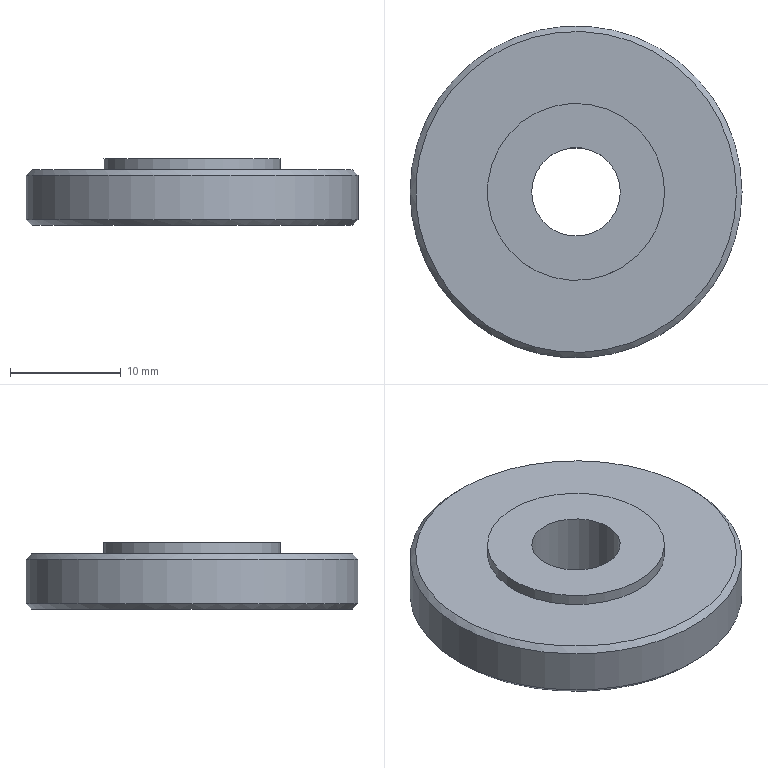Part | STEP file | Left | 1 solid | 8 faces | box 30 x 30 x 6 mm | volume 3410 mm3 | plane 3 | cylinder 3 | cone 2 | commonest cylinder face diameters 8 x1 16 x1 30 x1
STEP:
#1=CARTESIAN_POINT('',(0.,0.,0.));
#2=DIRECTION('',(0.,0.,1.));
#3=DIRECTION('',(1.,0.,0.));
#4=AXIS2_PLACEMENT_3D('',#1,#2,#3);
#5=CARTESIAN_POINT('',(14.5,0.,0.));
#6=VERTEX_POINT('',#5);
#7=CARTESIAN_POINT('',(0.,0.,0.));
#8=DIRECTION('',(0.,0.,-1.));
#9=DIRECTION('',(1.,0.,0.));
#10=AXIS2_PLACEMENT_3D('',#7,#8,#9);
#11=CIRCLE('',#10,14.5);
#12=CARTESIAN_POINT('',(0.,0.,0.));
#13=DIRECTION('',(0.,0.,-1.));
#14=DIRECTION('',(1.,0.,0.));
#15=AXIS2_PLACEMENT_3D('',#12,#13,#14);
#16=PLANE('',#15);
#17=CARTESIAN_POINT('',(0.,0.));
#18=DIRECTION('',(1.,0.));
#19=AXIS2_PLACEMENT_2D('',#17,#18);
#20=CIRCLE('',#19,14.5);
#21=(GEOMETRIC_REPRESENTATION_CONTEXT(2)PARAMETRIC_REPRESENTATION_CONTEXT()REPRESENTATION_CONTEXT('',''));
#22=DEFINITIONAL_REPRESENTATION('',(#20),#21);
#23=PCURVE('',#16,#22);
#24=CARTESIAN_POINT('',(0.,0.,0.5));
#25=DIRECTION('',(0.,0.,1.));
#26=DIRECTION('',(1.,0.,0.));
#27=AXIS2_PLACEMENT_3D('',#24,#25,#26);
#28=CONICAL_SURFACE('',#27,15.,0.7854);
#29=CARTESIAN_POINT('',(6.283,-0.5));
#30=DIRECTION('',(-1.,0.));
#31=VECTOR('',#30,1.);
#32=LINE('',#29,#31);
#33=(GEOMETRIC_REPRESENTATION_CONTEXT(2)PARAMETRIC_REPRESENTATION_CONTEXT()REPRESENTATION_CONTEXT('',''));
#34=DEFINITIONAL_REPRESENTATION('',(#32),#33);
#35=PCURVE('',#28,#34);
#36=SURFACE_CURVE('',#11,(#23,#35),.PCURVE_S1.);
#37=EDGE_CURVE('',#6,#6,#36,.T.);
#38=ORIENTED_EDGE('',*,*,#37,.F.);
#39=EDGE_LOOP('',(#38));
#40=FACE_BOUND('',#39,.F.);
#41=CARTESIAN_POINT('',(4.,0.,0.));
#42=VERTEX_POINT('',#41);
#43=CARTESIAN_POINT('',(0.,0.,0.));
#44=DIRECTION('',(0.,0.,-1.));
#45=DIRECTION('',(1.,0.,0.));
#46=AXIS2_PLACEMENT_3D('',#43,#44,#45);
#47=CIRCLE('',#46,4.);
#48=CARTESIAN_POINT('',(0.,0.));
#49=DIRECTION('',(1.,0.));
#50=AXIS2_PLACEMENT_2D('',#48,#49);
#51=CIRCLE('',#50,4.);
#52=(GEOMETRIC_REPRESENTATION_CONTEXT(2)PARAMETRIC_REPRESENTATION_CONTEXT()REPRESENTATION_CONTEXT('',''));
#53=DEFINITIONAL_REPRESENTATION('',(#51),#52);
#54=PCURVE('',#16,#53);
#55=CARTESIAN_POINT('',(0.,0.,6.));
#56=DIRECTION('',(0.,0.,-1.));
#57=DIRECTION('',(1.,0.,0.));
#58=AXIS2_PLACEMENT_3D('',#55,#56,#57);
#59=CYLINDRICAL_SURFACE('',#58,4.);
#60=CARTESIAN_POINT('',(0.,6.));
#61=DIRECTION('',(1.,0.));
#62=VECTOR('',#61,1.);
#63=LINE('',#60,#62);
#64=(GEOMETRIC_REPRESENTATION_CONTEXT(2)PARAMETRIC_REPRESENTATION_CONTEXT()REPRESENTATION_CONTEXT('',''));
#65=DEFINITIONAL_REPRESENTATION('',(#63),#64);
#66=PCURVE('',#59,#65);
#67=SURFACE_CURVE('',#47,(#54,#66),.PCURVE_S1.);
#68=EDGE_CURVE('',#42,#42,#67,.T.);
#69=ORIENTED_EDGE('',*,*,#68,.T.);
#70=EDGE_LOOP('',(#69));
#71=FACE_BOUND('',#70,.F.);
#72=ADVANCED_FACE('',(#40,#71),#16,.T.);
#73=CARTESIAN_POINT('',(15.,0.,0.5));
#74=VERTEX_POINT('',#73);
#75=CARTESIAN_POINT('',(0.,0.,0.5));
#76=DIRECTION('',(0.,0.,-1.));
#77=DIRECTION('',(1.,0.,0.));
#78=AXIS2_PLACEMENT_3D('',#75,#76,#77);
#79=CIRCLE('',#78,15.);
#80=CARTESIAN_POINT('',(6.283,0.));
#81=DIRECTION('',(-1.,0.));
#82=VECTOR('',#81,1.);
#83=LINE('',#80,#82);
#84=(GEOMETRIC_REPRESENTATION_CONTEXT(2)PARAMETRIC_REPRESENTATION_CONTEXT()REPRESENTATION_CONTEXT('',''));
#85=DEFINITIONAL_REPRESENTATION('',(#83),#84);
#86=PCURVE('',#28,#85);
#87=CARTESIAN_POINT('',(0.,0.,0.));
#88=DIRECTION('',(0.,0.,1.));
#89=DIRECTION('',(1.,0.,0.));
#90=AXIS2_PLACEMENT_3D('',#87,#88,#89);
#91=CYLINDRICAL_SURFACE('',#90,15.);
#92=CARTESIAN_POINT('',(6.283,0.5));
#93=DIRECTION('',(-1.,0.));
#94=VECTOR('',#93,1.);
#95=LINE('',#92,#94);
#96=(GEOMETRIC_REPRESENTATION_CONTEXT(2)PARAMETRIC_REPRESENTATION_CONTEXT()REPRESENTATION_CONTEXT('',''));
#97=DEFINITIONAL_REPRESENTATION('',(#95),#96);
#98=PCURVE('',#91,#97);
#99=SURFACE_CURVE('',#79,(#86,#98),.PCURVE_S1.);
#100=EDGE_CURVE('',#74,#74,#99,.T.);
#101=ORIENTED_EDGE('',*,*,#100,.T.);
#102=CARTESIAN_POINT('',(15.,0.,0.5));
#103=DIRECTION('',(0.7071,0.,0.7071));
#104=VECTOR('',#103,1.);
#105=LINE('',#102,#104);
#106=CARTESIAN_POINT('',(0.,0.));
#107=DIRECTION('',(0.,1.));
#108=VECTOR('',#107,1.);
#109=LINE('',#106,#108);
#110=(GEOMETRIC_REPRESENTATION_CONTEXT(2)PARAMETRIC_REPRESENTATION_CONTEXT()REPRESENTATION_CONTEXT('',''));
#111=DEFINITIONAL_REPRESENTATION('',(#109),#110);
#112=PCURVE('',#28,#111);
#113=CARTESIAN_POINT('',(6.283,0.));
#114=DIRECTION('',(0.,1.));
#115=VECTOR('',#114,1.);
#116=LINE('',#113,#115);
#117=(GEOMETRIC_REPRESENTATION_CONTEXT(2)PARAMETRIC_REPRESENTATION_CONTEXT()REPRESENTATION_CONTEXT('',''));
#118=DEFINITIONAL_REPRESENTATION('',(#116),#117);
#119=PCURVE('',#28,#118);
#120=SEAM_CURVE('',#105,(#112,#119),.PCURVE_S1.);
#121=EDGE_CURVE('',#6,#74,#120,.T.);
#122=ORIENTED_EDGE('',*,*,#121,.F.);
#123=ORIENTED_EDGE('',*,*,#37,.F.);
#124=ORIENTED_EDGE('',*,*,#121,.T.);
#125=EDGE_LOOP('',(#101,#122,#123,#124));
#126=FACE_BOUND('',#125,.T.);
#127=ADVANCED_FACE('',(#126),#28,.T.);
#128=CARTESIAN_POINT('',(4.,0.,6.));
#129=VERTEX_POINT('',#128);
#130=CARTESIAN_POINT('',(0.,0.,6.));
#131=DIRECTION('',(0.,0.,-1.));
#132=DIRECTION('',(1.,0.,0.));
#133=AXIS2_PLACEMENT_3D('',#130,#131,#132);
#134=CIRCLE('',#133,4.);
#135=CARTESIAN_POINT('',(0.,0.));
#136=DIRECTION('',(1.,0.));
#137=VECTOR('',#136,1.);
#138=LINE('',#135,#137);
#139=(GEOMETRIC_REPRESENTATION_CONTEXT(2)PARAMETRIC_REPRESENTATION_CONTEXT()REPRESENTATION_CONTEXT('',''));
#140=DEFINITIONAL_REPRESENTATION('',(#138),#139);
#141=PCURVE('',#59,#140);
#142=CARTESIAN_POINT('',(0.,0.,6.));
#143=DIRECTION('',(0.,0.,-1.));
#144=DIRECTION('',(1.,0.,0.));
#145=AXIS2_PLACEMENT_3D('',#142,#143,#144);
#146=PLANE('',#145);
#147=CARTESIAN_POINT('',(0.,0.));
#148=DIRECTION('',(1.,0.));
#149=AXIS2_PLACEMENT_2D('',#147,#148);
#150=CIRCLE('',#149,4.);
#151=(GEOMETRIC_REPRESENTATION_CONTEXT(2)PARAMETRIC_REPRESENTATION_CONTEXT()REPRESENTATION_CONTEXT('',''));
#152=DEFINITIONAL_REPRESENTATION('',(#150),#151);
#153=PCURVE('',#146,#152);
#154=SURFACE_CURVE('',#134,(#141,#153),.PCURVE_S1.);
#155=EDGE_CURVE('',#129,#129,#154,.T.);
#156=ORIENTED_EDGE('',*,*,#155,.T.);
#157=CARTESIAN_POINT('',(4.,0.,6.));
#158=DIRECTION('',(0.,0.,-1.));
#159=VECTOR('',#158,1.);
#160=LINE('',#157,#159);
#161=CARTESIAN_POINT('',(6.283,0.));
#162=DIRECTION('',(0.,1.));
#163=VECTOR('',#162,1.);
#164=LINE('',#161,#163);
#165=(GEOMETRIC_REPRESENTATION_CONTEXT(2)PARAMETRIC_REPRESENTATION_CONTEXT()REPRESENTATION_CONTEXT('',''));
#166=DEFINITIONAL_REPRESENTATION('',(#164),#165);
#167=PCURVE('',#59,#166);
#168=CARTESIAN_POINT('',(0.,0.));
#169=DIRECTION('',(0.,1.));
#170=VECTOR('',#169,1.);
#171=LINE('',#168,#170);
#172=(GEOMETRIC_REPRESENTATION_CONTEXT(2)PARAMETRIC_REPRESENTATION_CONTEXT()REPRESENTATION_CONTEXT('',''));
#173=DEFINITIONAL_REPRESENTATION('',(#171),#172);
#174=PCURVE('',#59,#173);
#175=SEAM_CURVE('',#160,(#167,#174),.PCURVE_S1.);
#176=EDGE_CURVE('',#129,#42,#175,.T.);
#177=ORIENTED_EDGE('',*,*,#176,.T.);
#178=ORIENTED_EDGE('',*,*,#68,.F.);
#179=ORIENTED_EDGE('',*,*,#176,.F.);
#180=EDGE_LOOP('',(#156,#177,#178,#179));
#181=FACE_BOUND('',#180,.F.);
#182=ADVANCED_FACE('',(#181),#59,.F.);
#183=CARTESIAN_POINT('',(15.,0.,4.5));
#184=VERTEX_POINT('',#183);
#185=CARTESIAN_POINT('',(0.,0.,4.5));
#186=DIRECTION('',(0.,0.,-1.));
#187=DIRECTION('',(1.,0.,0.));
#188=AXIS2_PLACEMENT_3D('',#185,#186,#187);
#189=CIRCLE('',#188,15.);
#190=CARTESIAN_POINT('',(6.283,4.5));
#191=DIRECTION('',(-1.,0.));
#192=VECTOR('',#191,1.);
#193=LINE('',#190,#192);
#194=(GEOMETRIC_REPRESENTATION_CONTEXT(2)PARAMETRIC_REPRESENTATION_CONTEXT()REPRESENTATION_CONTEXT('',''));
#195=DEFINITIONAL_REPRESENTATION('',(#193),#194);
#196=PCURVE('',#91,#195);
#197=CARTESIAN_POINT('',(0.,0.,4.5));
#198=DIRECTION('',(0.,0.,-1.));
#199=DIRECTION('',(1.,0.,0.));
#200=AXIS2_PLACEMENT_3D('',#197,#198,#199);
#201=CONICAL_SURFACE('',#200,15.,0.7854);
#202=CARTESIAN_POINT('',(0.,0.));
#203=DIRECTION('',(1.,0.));
#204=VECTOR('',#203,1.);
#205=LINE('',#202,#204);
#206=(GEOMETRIC_REPRESENTATION_CONTEXT(2)PARAMETRIC_REPRESENTATION_CONTEXT()REPRESENTATION_CONTEXT('',''));
#207=DEFINITIONAL_REPRESENTATION('',(#205),#206);
#208=PCURVE('',#201,#207);
#209=SURFACE_CURVE('',#189,(#196,#208),.PCURVE_S1.);
#210=EDGE_CURVE('',#184,#184,#209,.T.);
#211=ORIENTED_EDGE('',*,*,#210,.T.);
#212=CARTESIAN_POINT('',(15.,0.,0.));
#213=DIRECTION('',(0.,0.,1.));
#214=VECTOR('',#213,1.);
#215=LINE('',#212,#214);
#216=CARTESIAN_POINT('',(0.,0.));
#217=DIRECTION('',(0.,1.));
#218=VECTOR('',#217,1.);
#219=LINE('',#216,#218);
#220=(GEOMETRIC_REPRESENTATION_CONTEXT(2)PARAMETRIC_REPRESENTATION_CONTEXT()REPRESENTATION_CONTEXT('',''));
#221=DEFINITIONAL_REPRESENTATION('',(#219),#220);
#222=PCURVE('',#91,#221);
#223=CARTESIAN_POINT('',(6.283,0.));
#224=DIRECTION('',(0.,1.));
#225=VECTOR('',#224,1.);
#226=LINE('',#223,#225);
#227=(GEOMETRIC_REPRESENTATION_CONTEXT(2)PARAMETRIC_REPRESENTATION_CONTEXT()REPRESENTATION_CONTEXT('',''));
#228=DEFINITIONAL_REPRESENTATION('',(#226),#227);
#229=PCURVE('',#91,#228);
#230=SEAM_CURVE('',#215,(#222,#229),.PCURVE_S1.);
#231=EDGE_CURVE('',#74,#184,#230,.T.);
#232=ORIENTED_EDGE('',*,*,#231,.F.);
#233=ORIENTED_EDGE('',*,*,#100,.F.);
#234=ORIENTED_EDGE('',*,*,#231,.T.);
#235=EDGE_LOOP('',(#211,#232,#233,#234));
#236=FACE_BOUND('',#235,.T.);
#237=ADVANCED_FACE('',(#236),#91,.T.);
#238=CARTESIAN_POINT('',(8.,0.,6.));
#239=VERTEX_POINT('',#238);
#240=CARTESIAN_POINT('',(0.,0.,6.));
#241=DIRECTION('',(0.,0.,-1.));
#242=DIRECTION('',(1.,0.,0.));
#243=AXIS2_PLACEMENT_3D('',#240,#241,#242);
#244=CIRCLE('',#243,8.);
#245=CARTESIAN_POINT('',(0.,0.));
#246=DIRECTION('',(1.,0.));
#247=AXIS2_PLACEMENT_2D('',#245,#246);
#248=CIRCLE('',#247,8.);
#249=(GEOMETRIC_REPRESENTATION_CONTEXT(2)PARAMETRIC_REPRESENTATION_CONTEXT()REPRESENTATION_CONTEXT('',''));
#250=DEFINITIONAL_REPRESENTATION('',(#248),#249);
#251=PCURVE('',#146,#250);
#252=CARTESIAN_POINT('',(0.,0.,5.));
#253=DIRECTION('',(0.,0.,1.));
#254=DIRECTION('',(1.,0.,0.));
#255=AXIS2_PLACEMENT_3D('',#252,#253,#254);
#256=CYLINDRICAL_SURFACE('',#255,8.);
#257=CARTESIAN_POINT('',(6.283,1.));
#258=DIRECTION('',(-1.,0.));
#259=VECTOR('',#258,1.);
#260=LINE('',#257,#259);
#261=(GEOMETRIC_REPRESENTATION_CONTEXT(2)PARAMETRIC_REPRESENTATION_CONTEXT()REPRESENTATION_CONTEXT('',''));
#262=DEFINITIONAL_REPRESENTATION('',(#260),#261);
#263=PCURVE('',#256,#262);
#264=SURFACE_CURVE('',#244,(#251,#263),.PCURVE_S1.);
#265=EDGE_CURVE('',#239,#239,#264,.T.);
#266=ORIENTED_EDGE('',*,*,#265,.T.);
#267=EDGE_LOOP('',(#266));
#268=FACE_BOUND('',#267,.F.);
#269=ORIENTED_EDGE('',*,*,#155,.F.);
#270=EDGE_LOOP('',(#269));
#271=FACE_BOUND('',#270,.F.);
#272=ADVANCED_FACE('',(#268,#271),#146,.F.);
#273=CARTESIAN_POINT('',(14.5,0.,5.));
#274=VERTEX_POINT('',#273);
#275=CARTESIAN_POINT('',(0.,0.,5.));
#276=DIRECTION('',(0.,0.,-1.));
#277=DIRECTION('',(1.,0.,0.));
#278=AXIS2_PLACEMENT_3D('',#275,#276,#277);
#279=CIRCLE('',#278,14.5);
#280=CARTESIAN_POINT('',(0.,-0.5));
#281=DIRECTION('',(1.,0.));
#282=VECTOR('',#281,1.);
#283=LINE('',#280,#282);
#284=(GEOMETRIC_REPRESENTATION_CONTEXT(2)PARAMETRIC_REPRESENTATION_CONTEXT()REPRESENTATION_CONTEXT('',''));
#285=DEFINITIONAL_REPRESENTATION('',(#283),#284);
#286=PCURVE('',#201,#285);
#287=CARTESIAN_POINT('',(0.,0.,5.));
#288=DIRECTION('',(0.,0.,-1.));
#289=DIRECTION('',(1.,0.,0.));
#290=AXIS2_PLACEMENT_3D('',#287,#288,#289);
#291=PLANE('',#290);
#292=CARTESIAN_POINT('',(0.,0.));
#293=DIRECTION('',(1.,0.));
#294=AXIS2_PLACEMENT_2D('',#292,#293);
#295=CIRCLE('',#294,14.5);
#296=(GEOMETRIC_REPRESENTATION_CONTEXT(2)PARAMETRIC_REPRESENTATION_CONTEXT()REPRESENTATION_CONTEXT('',''));
#297=DEFINITIONAL_REPRESENTATION('',(#295),#296);
#298=PCURVE('',#291,#297);
#299=SURFACE_CURVE('',#279,(#286,#298),.PCURVE_S1.);
#300=EDGE_CURVE('',#274,#274,#299,.T.);
#301=ORIENTED_EDGE('',*,*,#300,.T.);
#302=CARTESIAN_POINT('',(15.,0.,4.5));
#303=DIRECTION('',(-0.7071,0.,0.7071));
#304=VECTOR('',#303,1.);
#305=LINE('',#302,#304);
#306=CARTESIAN_POINT('',(6.283,0.));
#307=DIRECTION('',(0.,-1.));
#308=VECTOR('',#307,1.);
#309=LINE('',#306,#308);
#310=(GEOMETRIC_REPRESENTATION_CONTEXT(2)PARAMETRIC_REPRESENTATION_CONTEXT()REPRESENTATION_CONTEXT('',''));
#311=DEFINITIONAL_REPRESENTATION('',(#309),#310);
#312=PCURVE('',#201,#311);
#313=CARTESIAN_POINT('',(0.,0.));
#314=DIRECTION('',(0.,-1.));
#315=VECTOR('',#314,1.);
#316=LINE('',#313,#315);
#317=(GEOMETRIC_REPRESENTATION_CONTEXT(2)PARAMETRIC_REPRESENTATION_CONTEXT()REPRESENTATION_CONTEXT('',''));
#318=DEFINITIONAL_REPRESENTATION('',(#316),#317);
#319=PCURVE('',#201,#318);
#320=SEAM_CURVE('',#305,(#312,#319),.PCURVE_S1.);
#321=EDGE_CURVE('',#184,#274,#320,.T.);
#322=ORIENTED_EDGE('',*,*,#321,.F.);
#323=ORIENTED_EDGE('',*,*,#210,.F.);
#324=ORIENTED_EDGE('',*,*,#321,.T.);
#325=EDGE_LOOP('',(#301,#322,#323,#324));
#326=FACE_BOUND('',#325,.T.);
#327=ADVANCED_FACE('',(#326),#201,.T.);
#328=CARTESIAN_POINT('',(8.,0.,5.));
#329=VERTEX_POINT('',#328);
#330=CARTESIAN_POINT('',(8.,0.,5.));
#331=DIRECTION('',(0.,0.,1.));
#332=VECTOR('',#331,1.);
#333=LINE('',#330,#332);
#334=CARTESIAN_POINT('',(6.283,0.));
#335=DIRECTION('',(0.,1.));
#336=VECTOR('',#335,1.);
#337=LINE('',#334,#336);
#338=(GEOMETRIC_REPRESENTATION_CONTEXT(2)PARAMETRIC_REPRESENTATION_CONTEXT()REPRESENTATION_CONTEXT('',''));
#339=DEFINITIONAL_REPRESENTATION('',(#337),#338);
#340=PCURVE('',#256,#339);
#341=CARTESIAN_POINT('',(0.,0.));
#342=DIRECTION('',(0.,1.));
#343=VECTOR('',#342,1.);
#344=LINE('',#341,#343);
#345=(GEOMETRIC_REPRESENTATION_CONTEXT(2)PARAMETRIC_REPRESENTATION_CONTEXT()REPRESENTATION_CONTEXT('',''));
#346=DEFINITIONAL_REPRESENTATION('',(#344),#345);
#347=PCURVE('',#256,#346);
#348=SEAM_CURVE('',#333,(#340,#347),.PCURVE_S1.);
#349=EDGE_CURVE('',#329,#239,#348,.T.);
#350=ORIENTED_EDGE('',*,*,#349,.T.);
#351=ORIENTED_EDGE('',*,*,#265,.T.);
#352=ORIENTED_EDGE('',*,*,#349,.F.);
#353=CARTESIAN_POINT('',(0.,0.,5.));
#354=DIRECTION('',(0.,0.,-1.));
#355=DIRECTION('',(1.,0.,0.));
#356=AXIS2_PLACEMENT_3D('',#353,#354,#355);
#357=CIRCLE('',#356,8.);
#358=CARTESIAN_POINT('',(6.283,0.));
#359=DIRECTION('',(-1.,0.));
#360=VECTOR('',#359,1.);
#361=LINE('',#358,#360);
#362=(GEOMETRIC_REPRESENTATION_CONTEXT(2)PARAMETRIC_REPRESENTATION_CONTEXT()REPRESENTATION_CONTEXT('',''));
#363=DEFINITIONAL_REPRESENTATION('',(#361),#362);
#364=PCURVE('',#256,#363);
#365=CARTESIAN_POINT('',(0.,0.));
#366=DIRECTION('',(1.,0.));
#367=AXIS2_PLACEMENT_2D('',#365,#366);
#368=CIRCLE('',#367,8.);
#369=(GEOMETRIC_REPRESENTATION_CONTEXT(2)PARAMETRIC_REPRESENTATION_CONTEXT()REPRESENTATION_CONTEXT('',''));
#370=DEFINITIONAL_REPRESENTATION('',(#368),#369);
#371=PCURVE('',#291,#370);
#372=SURFACE_CURVE('',#357,(#364,#371),.PCURVE_S1.);
#373=EDGE_CURVE('',#329,#329,#372,.T.);
#374=ORIENTED_EDGE('',*,*,#373,.F.);
#375=EDGE_LOOP('',(#350,#351,#352,#374));
#376=FACE_BOUND('',#375,.T.);
#377=ADVANCED_FACE('',(#376),#256,.T.);
#378=ORIENTED_EDGE('',*,*,#300,.T.);
#379=EDGE_LOOP('',(#378));
#380=FACE_BOUND('',#379,.F.);
#381=ORIENTED_EDGE('',*,*,#373,.F.);
#382=EDGE_LOOP('',(#381));
#383=FACE_BOUND('',#382,.F.);
#384=ADVANCED_FACE('',(#380,#383),#291,.F.);
#385=CLOSED_SHELL('',(#72,#127,#182,#237,#272,#327,#377,#384));
#386=MANIFOLD_SOLID_BREP('',#385);
#387=(LENGTH_UNIT()NAMED_UNIT(*)SI_UNIT(.MILLI.,.METRE.));
#388=UNCERTAINTY_MEASURE_WITH_UNIT(LENGTH_MEASURE(0.0000001),#387,'','');
#389=(NAMED_UNIT(*)PLANE_ANGLE_UNIT()SI_UNIT($,.RADIAN.));
#390=(NAMED_UNIT(*)SI_UNIT($,.STERADIAN.)SOLID_ANGLE_UNIT());
#391=(GEOMETRIC_REPRESENTATION_CONTEXT(3)GLOBAL_UNCERTAINTY_ASSIGNED_CONTEXT((#388))GLOBAL_UNIT_ASSIGNED_CONTEXT((#387,#389,#390))REPRESENTATION_CONTEXT('',''));
#392=ADVANCED_BREP_SHAPE_REPRESENTATION('',(#4,#386),#391);